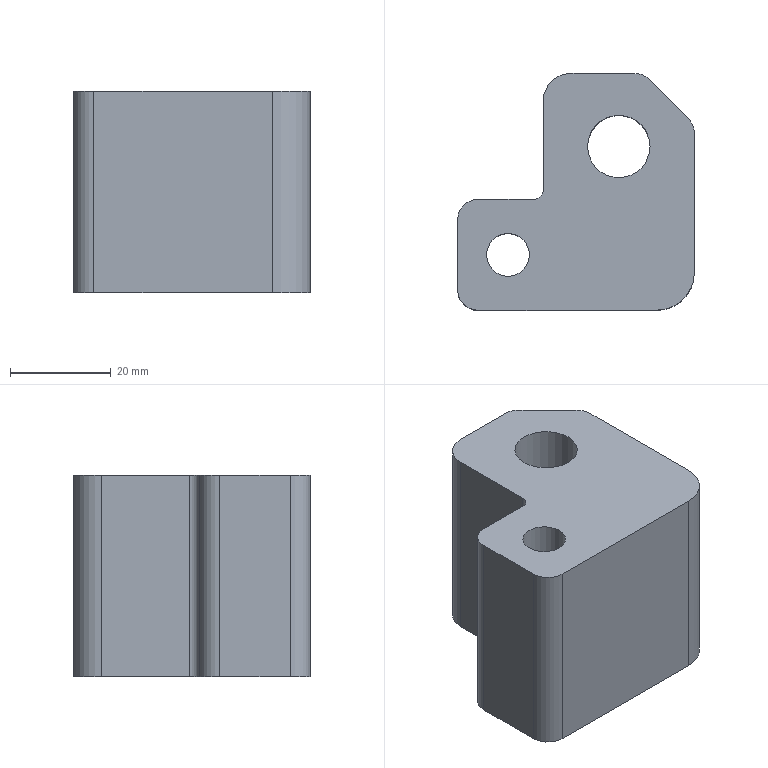Part | NX | features PS-7 2 | 1 solid | 20 faces | box 47 x 47 x 40 mm | volume 59988 mm3 | plane 10 | cylinder 10 | commonest cylinder face diameters 8 x4 4 x1 8.5 x1 11 x1 12.4 x1 14.5 x1
STEP:
#1=CARTESIAN_POINT('',(2465.297,-809.449,860.716));
#2=VERTEX_POINT('',#1);
#3=CARTESIAN_POINT('',(2459.097,-809.449,860.716));
#4=DIRECTION('',(0.,0.,1.));
#5=DIRECTION('',(1.,0.,0.));
#6=AXIS2_PLACEMENT_3D('',#3,#4,#5);
#7=CIRCLE('',#6,6.2);
#8=EDGE_CURVE('',#2,#2,#7,.T.);
#9=ORIENTED_EDGE('',*,*,#8,.T.);
#10=EDGE_LOOP('',(#9));
#11=FACE_BOUND('',#10,.T.);
#12=CARTESIAN_POINT('',(2444.347,-830.949,860.716));
#13=VERTEX_POINT('',#12);
#14=CARTESIAN_POINT('',(2437.097,-830.949,860.716));
#15=DIRECTION('',(0.,0.,1.));
#16=DIRECTION('',(1.,0.,0.));
#17=AXIS2_PLACEMENT_3D('',#14,#15,#16);
#18=CIRCLE('',#17,7.25);
#19=EDGE_CURVE('',#13,#13,#18,.T.);
#20=ORIENTED_EDGE('',*,*,#19,.T.);
#21=EDGE_LOOP('',(#20));
#22=FACE_BOUND('',#21,.T.);
#23=CARTESIAN_POINT('',(2474.097,-834.449,860.716));
#24=VERTEX_POINT('',#23);
#25=CARTESIAN_POINT('',(2466.597,-841.949,860.716));
#26=VERTEX_POINT('',#25);
#27=CARTESIAN_POINT('',(2466.597,-834.449,860.716));
#28=DIRECTION('',(0.,0.,1.));
#29=DIRECTION('',(1.,0.,0.));
#30=AXIS2_PLACEMENT_3D('',#27,#28,#29);
#31=CIRCLE('',#30,7.5);
#32=EDGE_CURVE('',#24,#26,#31,.F.);
#33=ORIENTED_EDGE('',*,*,#32,.T.);
#34=CARTESIAN_POINT('',(2431.097,-841.949,860.716));
#35=VERTEX_POINT('',#34);
#36=CARTESIAN_POINT('',(0.,-841.949,860.716));
#37=DIRECTION('',(1.,0.,0.));
#38=VECTOR('',#37,1000.);
#39=LINE('',#36,#38);
#40=EDGE_CURVE('',#35,#26,#39,.T.);
#41=ORIENTED_EDGE('',*,*,#40,.F.);
#42=CARTESIAN_POINT('',(2427.097,-837.949,860.716));
#43=VERTEX_POINT('',#42);
#44=CARTESIAN_POINT('',(2431.097,-837.949,860.716));
#45=DIRECTION('',(0.,0.,1.));
#46=DIRECTION('',(1.,0.,0.));
#47=AXIS2_PLACEMENT_3D('',#44,#45,#46);
#48=CIRCLE('',#47,4.);
#49=EDGE_CURVE('',#43,#35,#48,.T.);
#50=ORIENTED_EDGE('',*,*,#49,.F.);
#51=CARTESIAN_POINT('',(2427.097,-823.949,860.716));
#52=VERTEX_POINT('',#51);
#53=CARTESIAN_POINT('',(2427.097,-800.449,860.716));
#54=DIRECTION('',(0.,1.,0.));
#55=VECTOR('',#54,1000.);
#56=LINE('',#53,#55);
#57=EDGE_CURVE('',#43,#52,#56,.T.);
#58=ORIENTED_EDGE('',*,*,#57,.T.);
#59=CARTESIAN_POINT('',(2431.097,-819.949,860.716));
#60=VERTEX_POINT('',#59);
#61=CARTESIAN_POINT('',(2431.097,-823.949,860.716));
#62=DIRECTION('',(0.,0.,1.));
#63=DIRECTION('',(1.,0.,0.));
#64=AXIS2_PLACEMENT_3D('',#61,#62,#63);
#65=CIRCLE('',#64,4.);
#66=EDGE_CURVE('',#52,#60,#65,.F.);
#67=ORIENTED_EDGE('',*,*,#66,.T.);
#68=CARTESIAN_POINT('',(2442.097,-819.949,860.716));
#69=VERTEX_POINT('',#68);
#70=CARTESIAN_POINT('',(2437.597,-819.949,860.716));
#71=DIRECTION('',(-1.,0.,0.));
#72=VECTOR('',#71,1000.);
#73=LINE('',#70,#72);
#74=EDGE_CURVE('',#69,#60,#73,.T.);
#75=ORIENTED_EDGE('',*,*,#74,.F.);
#76=CARTESIAN_POINT('',(2444.097,-817.949,860.716));
#77=VERTEX_POINT('',#76);
#78=CARTESIAN_POINT('',(2442.097,-817.949,860.716));
#79=DIRECTION('',(0.,0.,1.));
#80=DIRECTION('',(1.,0.,0.));
#81=AXIS2_PLACEMENT_3D('',#78,#79,#80);
#82=CIRCLE('',#81,2.);
#83=EDGE_CURVE('',#77,#69,#82,.F.);
#84=ORIENTED_EDGE('',*,*,#83,.F.);
#85=CARTESIAN_POINT('',(2444.097,-800.449,860.716));
#86=VERTEX_POINT('',#85);
#87=CARTESIAN_POINT('',(2444.097,-800.449,860.716));
#88=DIRECTION('',(0.,1.,0.));
#89=VECTOR('',#88,1000.);
#90=LINE('',#87,#89);
#91=EDGE_CURVE('',#77,#86,#90,.T.);
#92=ORIENTED_EDGE('',*,*,#91,.T.);
#93=CARTESIAN_POINT('',(2449.597,-794.949,860.716));
#94=VERTEX_POINT('',#93);
#95=CARTESIAN_POINT('',(2449.597,-800.449,860.716));
#96=DIRECTION('',(0.,0.,1.));
#97=DIRECTION('',(1.,0.,0.));
#98=AXIS2_PLACEMENT_3D('',#95,#96,#97);
#99=CIRCLE('',#98,5.5);
#100=EDGE_CURVE('',#86,#94,#99,.F.);
#101=ORIENTED_EDGE('',*,*,#100,.T.);
#102=CARTESIAN_POINT('',(2462.269,-794.949,860.716));
#103=VERTEX_POINT('',#102);
#104=CARTESIAN_POINT('',(0.,-794.949,860.716));
#105=DIRECTION('',(-1.,0.,0.));
#106=VECTOR('',#105,1000.);
#107=LINE('',#104,#106);
#108=EDGE_CURVE('',#103,#94,#107,.T.);
#109=ORIENTED_EDGE('',*,*,#108,.F.);
#110=CARTESIAN_POINT('',(2465.097,-796.12,860.716));
#111=VERTEX_POINT('',#110);
#112=CARTESIAN_POINT('',(2462.269,-798.949,860.716));
#113=DIRECTION('',(0.,0.,1.));
#114=DIRECTION('',(1.,0.,0.));
#115=AXIS2_PLACEMENT_3D('',#112,#113,#114);
#116=CIRCLE('',#115,4.);
#117=EDGE_CURVE('',#103,#111,#116,.F.);
#118=ORIENTED_EDGE('',*,*,#117,.T.);
#119=CARTESIAN_POINT('',(2472.926,-803.949,860.716));
#120=VERTEX_POINT('',#119);
#121=CARTESIAN_POINT('',(834.488,834.488,860.716));
#122=DIRECTION('',(-0.7071,0.7071,0.));
#123=VECTOR('',#122,1000.);
#124=LINE('',#121,#123);
#125=EDGE_CURVE('',#120,#111,#124,.T.);
#126=ORIENTED_EDGE('',*,*,#125,.F.);
#127=CARTESIAN_POINT('',(2474.097,-806.777,860.716));
#128=VERTEX_POINT('',#127);
#129=CARTESIAN_POINT('',(2470.097,-806.777,860.716));
#130=DIRECTION('',(0.,0.,1.));
#131=DIRECTION('',(1.,0.,0.));
#132=AXIS2_PLACEMENT_3D('',#129,#130,#131);
#133=CIRCLE('',#132,4.);
#134=EDGE_CURVE('',#128,#120,#133,.T.);
#135=ORIENTED_EDGE('',*,*,#134,.F.);
#136=CARTESIAN_POINT('',(2474.097,-834.449,860.716));
#137=DIRECTION('',(0.,-1.,0.));
#138=VECTOR('',#137,1000.);
#139=LINE('',#136,#138);
#140=EDGE_CURVE('',#128,#24,#139,.T.);
#141=ORIENTED_EDGE('',*,*,#140,.T.);
#142=EDGE_LOOP('',(#33,#41,#50,#58,#67,#75,#84,#92,#101,#109,#118,#126,#135,#141));
#143=FACE_BOUND('',#142,.T.);
#144=CARTESIAN_POINT('',(0.,0.,860.716));
#145=DIRECTION('',(0.,0.,1.));
#146=DIRECTION('',(1.,0.,0.));
#147=AXIS2_PLACEMENT_3D('',#144,#145,#146);
#148=PLANE('',#147);
#149=ADVANCED_FACE('',(#11,#22,#143),#148,.F.);
#150=ORIENTED_EDGE('',*,*,#91,.F.);
#151=CARTESIAN_POINT('',(2444.097,-817.949,900.716));
#152=VERTEX_POINT('',#151);
#153=CARTESIAN_POINT('',(2444.097,-817.949,830.716));
#154=DIRECTION('',(0.,0.,1.));
#155=VECTOR('',#154,1000.);
#156=LINE('',#153,#155);
#157=EDGE_CURVE('',#77,#152,#156,.T.);
#158=ORIENTED_EDGE('',*,*,#157,.T.);
#159=CARTESIAN_POINT('',(2444.097,-800.449,900.716));
#160=VERTEX_POINT('',#159);
#161=CARTESIAN_POINT('',(2444.097,-800.449,900.716));
#162=DIRECTION('',(0.,1.,0.));
#163=VECTOR('',#162,1000.);
#164=LINE('',#161,#163);
#165=EDGE_CURVE('',#152,#160,#164,.T.);
#166=ORIENTED_EDGE('',*,*,#165,.T.);
#167=CARTESIAN_POINT('',(2444.097,-800.449,830.716));
#168=DIRECTION('',(0.,0.,1.));
#169=VECTOR('',#168,1000.);
#170=LINE('',#167,#169);
#171=EDGE_CURVE('',#160,#86,#170,.F.);
#172=ORIENTED_EDGE('',*,*,#171,.T.);
#173=EDGE_LOOP('',(#150,#158,#166,#172));
#174=FACE_BOUND('',#173,.T.);
#175=CARTESIAN_POINT('',(2444.097,-800.449,830.716));
#176=DIRECTION('',(-1.,0.,0.));
#177=DIRECTION('',(0.,0.,1.));
#178=AXIS2_PLACEMENT_3D('',#175,#176,#177);
#179=PLANE('',#178);
#180=ADVANCED_FACE('',(#174),#179,.T.);
#181=CARTESIAN_POINT('',(2431.097,-841.949,900.716));
#182=VERTEX_POINT('',#181);
#183=CARTESIAN_POINT('',(2466.597,-841.949,900.716));
#184=VERTEX_POINT('',#183);
#185=CARTESIAN_POINT('',(0.,-841.949,900.716));
#186=DIRECTION('',(1.,0.,0.));
#187=VECTOR('',#186,1000.);
#188=LINE('',#185,#187);
#189=EDGE_CURVE('',#182,#184,#188,.T.);
#190=ORIENTED_EDGE('',*,*,#189,.F.);
#191=CARTESIAN_POINT('',(2431.097,-841.949,830.716));
#192=DIRECTION('',(0.,0.,-1.));
#193=VECTOR('',#192,1000.);
#194=LINE('',#191,#193);
#195=EDGE_CURVE('',#182,#35,#194,.T.);
#196=ORIENTED_EDGE('',*,*,#195,.T.);
#197=ORIENTED_EDGE('',*,*,#40,.T.);
#198=CARTESIAN_POINT('',(2466.597,-841.949,830.716));
#199=DIRECTION('',(0.,0.,1.));
#200=VECTOR('',#199,1000.);
#201=LINE('',#198,#200);
#202=EDGE_CURVE('',#184,#26,#201,.F.);
#203=ORIENTED_EDGE('',*,*,#202,.F.);
#204=EDGE_LOOP('',(#190,#196,#197,#203));
#205=FACE_BOUND('',#204,.T.);
#206=CARTESIAN_POINT('',(2449.597,-841.949,830.716));
#207=DIRECTION('',(0.,-1.,0.));
#208=DIRECTION('',(0.,0.,-1.));
#209=AXIS2_PLACEMENT_3D('',#206,#207,#208);
#210=PLANE('',#209);
#211=ADVANCED_FACE('',(#205),#210,.T.);
#212=ORIENTED_EDGE('',*,*,#202,.T.);
#213=ORIENTED_EDGE('',*,*,#32,.F.);
#214=CARTESIAN_POINT('',(2474.097,-834.449,900.716));
#215=VERTEX_POINT('',#214);
#216=CARTESIAN_POINT('',(2474.097,-834.449,830.716));
#217=DIRECTION('',(0.,0.,-1.));
#218=VECTOR('',#217,1000.);
#219=LINE('',#216,#218);
#220=EDGE_CURVE('',#215,#24,#219,.T.);
#221=ORIENTED_EDGE('',*,*,#220,.F.);
#222=CARTESIAN_POINT('',(2466.597,-834.449,900.716));
#223=DIRECTION('',(0.,0.,1.));
#224=DIRECTION('',(1.,0.,0.));
#225=AXIS2_PLACEMENT_3D('',#222,#223,#224);
#226=CIRCLE('',#225,7.5);
#227=EDGE_CURVE('',#215,#184,#226,.F.);
#228=ORIENTED_EDGE('',*,*,#227,.T.);
#229=EDGE_LOOP('',(#212,#213,#221,#228));
#230=FACE_BOUND('',#229,.T.);
#231=CARTESIAN_POINT('',(2466.597,-834.449,830.716));
#232=DIRECTION('',(0.,0.,1.));
#233=DIRECTION('',(1.,0.,0.));
#234=AXIS2_PLACEMENT_3D('',#231,#232,#233);
#235=CYLINDRICAL_SURFACE('',#234,7.5);
#236=ADVANCED_FACE('',(#230),#235,.T.);
#237=ORIENTED_EDGE('',*,*,#220,.T.);
#238=ORIENTED_EDGE('',*,*,#140,.F.);
#239=CARTESIAN_POINT('',(2474.097,-806.777,900.716));
#240=VERTEX_POINT('',#239);
#241=CARTESIAN_POINT('',(2474.097,-806.777,830.716));
#242=DIRECTION('',(0.,0.,1.));
#243=VECTOR('',#242,1000.);
#244=LINE('',#241,#243);
#245=EDGE_CURVE('',#240,#128,#244,.F.);
#246=ORIENTED_EDGE('',*,*,#245,.F.);
#247=CARTESIAN_POINT('',(2474.097,-834.449,900.716));
#248=DIRECTION('',(0.,-1.,0.));
#249=VECTOR('',#248,1000.);
#250=LINE('',#247,#249);
#251=EDGE_CURVE('',#240,#215,#250,.T.);
#252=ORIENTED_EDGE('',*,*,#251,.T.);
#253=EDGE_LOOP('',(#237,#238,#246,#252));
#254=FACE_BOUND('',#253,.T.);
#255=CARTESIAN_POINT('',(2474.097,-834.449,830.716));
#256=DIRECTION('',(1.,0.,0.));
#257=DIRECTION('',(0.,0.,-1.));
#258=AXIS2_PLACEMENT_3D('',#255,#256,#257);
#259=PLANE('',#258);
#260=ADVANCED_FACE('',(#254),#259,.T.);
#261=ORIENTED_EDGE('',*,*,#245,.T.);
#262=ORIENTED_EDGE('',*,*,#134,.T.);
#263=CARTESIAN_POINT('',(2472.926,-803.949,900.716));
#264=VERTEX_POINT('',#263);
#265=CARTESIAN_POINT('',(2472.926,-803.949,830.716));
#266=DIRECTION('',(0.,0.,1.));
#267=VECTOR('',#266,1000.);
#268=LINE('',#265,#267);
#269=EDGE_CURVE('',#264,#120,#268,.F.);
#270=ORIENTED_EDGE('',*,*,#269,.F.);
#271=CARTESIAN_POINT('',(2470.097,-806.777,900.716));
#272=DIRECTION('',(0.,0.,1.));
#273=DIRECTION('',(1.,0.,0.));
#274=AXIS2_PLACEMENT_3D('',#271,#272,#273);
#275=CIRCLE('',#274,4.);
#276=EDGE_CURVE('',#264,#240,#275,.F.);
#277=ORIENTED_EDGE('',*,*,#276,.T.);
#278=EDGE_LOOP('',(#261,#262,#270,#277));
#279=FACE_BOUND('',#278,.T.);
#280=CARTESIAN_POINT('',(2470.097,-806.777,830.716));
#281=DIRECTION('',(0.,0.,1.));
#282=DIRECTION('',(1.,0.,0.));
#283=AXIS2_PLACEMENT_3D('',#280,#281,#282);
#284=CYLINDRICAL_SURFACE('',#283,4.);
#285=ADVANCED_FACE('',(#279),#284,.T.);
#286=ORIENTED_EDGE('',*,*,#269,.T.);
#287=ORIENTED_EDGE('',*,*,#125,.T.);
#288=CARTESIAN_POINT('',(2465.097,-796.12,900.716));
#289=VERTEX_POINT('',#288);
#290=CARTESIAN_POINT('',(2465.097,-796.12,830.716));
#291=DIRECTION('',(0.,0.,1.));
#292=VECTOR('',#291,1000.);
#293=LINE('',#290,#292);
#294=EDGE_CURVE('',#289,#111,#293,.F.);
#295=ORIENTED_EDGE('',*,*,#294,.F.);
#296=CARTESIAN_POINT('',(2472.926,-803.949,900.716));
#297=DIRECTION('',(0.7071,-0.7071,0.));
#298=VECTOR('',#297,1000.);
#299=LINE('',#296,#298);
#300=EDGE_CURVE('',#289,#264,#299,.T.);
#301=ORIENTED_EDGE('',*,*,#300,.T.);
#302=EDGE_LOOP('',(#286,#287,#295,#301));
#303=FACE_BOUND('',#302,.T.);
#304=CARTESIAN_POINT('',(2472.926,-803.949,830.716));
#305=DIRECTION('',(0.7071,0.7071,0.));
#306=DIRECTION('',(-0.7071,0.7071,0.));
#307=AXIS2_PLACEMENT_3D('',#304,#305,#306);
#308=PLANE('',#307);
#309=ADVANCED_FACE('',(#303),#308,.T.);
#310=ORIENTED_EDGE('',*,*,#294,.T.);
#311=ORIENTED_EDGE('',*,*,#117,.F.);
#312=CARTESIAN_POINT('',(2462.269,-794.949,900.716));
#313=VERTEX_POINT('',#312);
#314=CARTESIAN_POINT('',(2462.269,-794.949,830.716));
#315=DIRECTION('',(0.,0.,1.));
#316=VECTOR('',#315,1000.);
#317=LINE('',#314,#316);
#318=EDGE_CURVE('',#313,#103,#317,.F.);
#319=ORIENTED_EDGE('',*,*,#318,.F.);
#320=CARTESIAN_POINT('',(2462.269,-798.949,900.716));
#321=DIRECTION('',(0.,0.,1.));
#322=DIRECTION('',(1.,0.,0.));
#323=AXIS2_PLACEMENT_3D('',#320,#321,#322);
#324=CIRCLE('',#323,4.);
#325=EDGE_CURVE('',#313,#289,#324,.F.);
#326=ORIENTED_EDGE('',*,*,#325,.T.);
#327=EDGE_LOOP('',(#310,#311,#319,#326));
#328=FACE_BOUND('',#327,.T.);
#329=CARTESIAN_POINT('',(2462.269,-798.949,830.716));
#330=DIRECTION('',(0.,0.,1.));
#331=DIRECTION('',(1.,0.,0.));
#332=AXIS2_PLACEMENT_3D('',#329,#330,#331);
#333=CYLINDRICAL_SURFACE('',#332,4.);
#334=ADVANCED_FACE('',(#328),#333,.T.);
#335=ORIENTED_EDGE('',*,*,#318,.T.);
#336=ORIENTED_EDGE('',*,*,#108,.T.);
#337=CARTESIAN_POINT('',(2449.597,-794.949,900.716));
#338=VERTEX_POINT('',#337);
#339=CARTESIAN_POINT('',(2449.597,-794.949,830.716));
#340=DIRECTION('',(0.,0.,1.));
#341=VECTOR('',#340,1000.);
#342=LINE('',#339,#341);
#343=EDGE_CURVE('',#338,#94,#342,.F.);
#344=ORIENTED_EDGE('',*,*,#343,.F.);
#345=CARTESIAN_POINT('',(2462.269,-794.949,900.716));
#346=DIRECTION('',(1.,0.,0.));
#347=VECTOR('',#346,1000.);
#348=LINE('',#345,#347);
#349=EDGE_CURVE('',#338,#313,#348,.T.);
#350=ORIENTED_EDGE('',*,*,#349,.T.);
#351=EDGE_LOOP('',(#335,#336,#344,#350));
#352=FACE_BOUND('',#351,.T.);
#353=CARTESIAN_POINT('',(2462.269,-794.949,830.716));
#354=DIRECTION('',(0.,1.,0.));
#355=DIRECTION('',(0.,0.,1.));
#356=AXIS2_PLACEMENT_3D('',#353,#354,#355);
#357=PLANE('',#356);
#358=ADVANCED_FACE('',(#352),#357,.T.);
#359=ORIENTED_EDGE('',*,*,#343,.T.);
#360=ORIENTED_EDGE('',*,*,#100,.F.);
#361=ORIENTED_EDGE('',*,*,#171,.F.);
#362=CARTESIAN_POINT('',(2449.597,-800.449,900.716));
#363=DIRECTION('',(0.,0.,1.));
#364=DIRECTION('',(1.,0.,0.));
#365=AXIS2_PLACEMENT_3D('',#362,#363,#364);
#366=CIRCLE('',#365,5.5);
#367=EDGE_CURVE('',#160,#338,#366,.F.);
#368=ORIENTED_EDGE('',*,*,#367,.T.);
#369=EDGE_LOOP('',(#359,#360,#361,#368));
#370=FACE_BOUND('',#369,.T.);
#371=CARTESIAN_POINT('',(2449.597,-800.449,830.716));
#372=DIRECTION('',(0.,0.,1.));
#373=DIRECTION('',(1.,0.,0.));
#374=AXIS2_PLACEMENT_3D('',#371,#372,#373);
#375=CYLINDRICAL_SURFACE('',#374,5.5);
#376=ADVANCED_FACE('',(#370),#375,.T.);
#377=ORIENTED_EDGE('',*,*,#57,.F.);
#378=CARTESIAN_POINT('',(2427.097,-837.949,900.716));
#379=VERTEX_POINT('',#378);
#380=CARTESIAN_POINT('',(2427.097,-837.949,830.716));
#381=DIRECTION('',(0.,0.,1.));
#382=VECTOR('',#381,1000.);
#383=LINE('',#380,#382);
#384=EDGE_CURVE('',#43,#379,#383,.T.);
#385=ORIENTED_EDGE('',*,*,#384,.T.);
#386=CARTESIAN_POINT('',(2427.097,-823.949,900.716));
#387=VERTEX_POINT('',#386);
#388=CARTESIAN_POINT('',(2427.097,-800.449,900.716));
#389=DIRECTION('',(0.,1.,0.));
#390=VECTOR('',#389,1000.);
#391=LINE('',#388,#390);
#392=EDGE_CURVE('',#379,#387,#391,.T.);
#393=ORIENTED_EDGE('',*,*,#392,.T.);
#394=CARTESIAN_POINT('',(2427.097,-823.949,830.716));
#395=DIRECTION('',(0.,0.,1.));
#396=VECTOR('',#395,1000.);
#397=LINE('',#394,#396);
#398=EDGE_CURVE('',#387,#52,#397,.F.);
#399=ORIENTED_EDGE('',*,*,#398,.T.);
#400=EDGE_LOOP('',(#377,#385,#393,#399));
#401=FACE_BOUND('',#400,.T.);
#402=CARTESIAN_POINT('',(2427.097,-800.449,830.716));
#403=DIRECTION('',(-1.,0.,0.));
#404=DIRECTION('',(0.,0.,1.));
#405=AXIS2_PLACEMENT_3D('',#402,#403,#404);
#406=PLANE('',#405);
#407=ADVANCED_FACE('',(#401),#406,.T.);
#408=CARTESIAN_POINT('',(2431.097,-819.949,900.716));
#409=VERTEX_POINT('',#408);
#410=CARTESIAN_POINT('',(2442.097,-819.949,900.716));
#411=VERTEX_POINT('',#410);
#412=CARTESIAN_POINT('',(0.,-819.949,900.716));
#413=DIRECTION('',(1.,0.,0.));
#414=VECTOR('',#413,1000.);
#415=LINE('',#412,#414);
#416=EDGE_CURVE('',#409,#411,#415,.T.);
#417=ORIENTED_EDGE('',*,*,#416,.T.);
#418=CARTESIAN_POINT('',(2442.097,-819.949,875.716));
#419=DIRECTION('',(0.,0.,-1.));
#420=VECTOR('',#419,1000.);
#421=LINE('',#418,#420);
#422=EDGE_CURVE('',#411,#69,#421,.T.);
#423=ORIENTED_EDGE('',*,*,#422,.T.);
#424=ORIENTED_EDGE('',*,*,#74,.T.);
#425=CARTESIAN_POINT('',(2431.097,-819.949,875.716));
#426=DIRECTION('',(0.,0.,-1.));
#427=VECTOR('',#426,1000.);
#428=LINE('',#425,#427);
#429=EDGE_CURVE('',#60,#409,#428,.F.);
#430=ORIENTED_EDGE('',*,*,#429,.T.);
#431=EDGE_LOOP('',(#417,#423,#424,#430));
#432=FACE_BOUND('',#431,.T.);
#433=CARTESIAN_POINT('',(2437.597,-819.949,875.716));
#434=DIRECTION('',(0.,-1.,0.));
#435=DIRECTION('',(0.,0.,-1.));
#436=AXIS2_PLACEMENT_3D('',#433,#434,#435);
#437=PLANE('',#436);
#438=ADVANCED_FACE('',(#432),#437,.F.);
#439=ORIENTED_EDGE('',*,*,#83,.T.);
#440=ORIENTED_EDGE('',*,*,#422,.F.);
#441=CARTESIAN_POINT('',(2442.097,-817.949,900.716));
#442=DIRECTION('',(0.,0.,1.));
#443=DIRECTION('',(1.,0.,0.));
#444=AXIS2_PLACEMENT_3D('',#441,#442,#443);
#445=CIRCLE('',#444,2.);
#446=EDGE_CURVE('',#152,#411,#445,.F.);
#447=ORIENTED_EDGE('',*,*,#446,.F.);
#448=ORIENTED_EDGE('',*,*,#157,.F.);
#449=EDGE_LOOP('',(#439,#440,#447,#448));
#450=FACE_BOUND('',#449,.T.);
#451=CARTESIAN_POINT('',(2442.097,-817.949,830.716));
#452=DIRECTION('',(0.,0.,1.));
#453=DIRECTION('',(1.,0.,0.));
#454=AXIS2_PLACEMENT_3D('',#451,#452,#453);
#455=CYLINDRICAL_SURFACE('',#454,2.);
#456=ADVANCED_FACE('',(#450),#455,.F.);
#457=CARTESIAN_POINT('',(2431.097,-837.949,900.716));
#458=DIRECTION('',(0.,0.,1.));
#459=DIRECTION('',(1.,0.,0.));
#460=AXIS2_PLACEMENT_3D('',#457,#458,#459);
#461=CIRCLE('',#460,4.);
#462=EDGE_CURVE('',#379,#182,#461,.T.);
#463=ORIENTED_EDGE('',*,*,#462,.F.);
#464=ORIENTED_EDGE('',*,*,#384,.F.);
#465=ORIENTED_EDGE('',*,*,#49,.T.);
#466=ORIENTED_EDGE('',*,*,#195,.F.);
#467=EDGE_LOOP('',(#463,#464,#465,#466));
#468=FACE_BOUND('',#467,.T.);
#469=CARTESIAN_POINT('',(2431.097,-837.949,830.716));
#470=DIRECTION('',(0.,0.,-1.));
#471=DIRECTION('',(-1.,0.,0.));
#472=AXIS2_PLACEMENT_3D('',#469,#470,#471);
#473=CYLINDRICAL_SURFACE('',#472,4.);
#474=ADVANCED_FACE('',(#468),#473,.T.);
#475=ORIENTED_EDGE('',*,*,#66,.F.);
#476=ORIENTED_EDGE('',*,*,#398,.F.);
#477=CARTESIAN_POINT('',(2431.097,-823.949,900.716));
#478=DIRECTION('',(0.,0.,1.));
#479=DIRECTION('',(1.,0.,0.));
#480=AXIS2_PLACEMENT_3D('',#477,#478,#479);
#481=CIRCLE('',#480,4.);
#482=EDGE_CURVE('',#387,#409,#481,.F.);
#483=ORIENTED_EDGE('',*,*,#482,.T.);
#484=ORIENTED_EDGE('',*,*,#429,.F.);
#485=EDGE_LOOP('',(#475,#476,#483,#484));
#486=FACE_BOUND('',#485,.T.);
#487=CARTESIAN_POINT('',(2431.097,-823.949,875.716));
#488=DIRECTION('',(0.,0.,-1.));
#489=DIRECTION('',(-1.,0.,0.));
#490=AXIS2_PLACEMENT_3D('',#487,#488,#489);
#491=CYLINDRICAL_SURFACE('',#490,4.);
#492=ADVANCED_FACE('',(#486),#491,.T.);
#493=CARTESIAN_POINT('',(2465.297,-809.449,900.716));
#494=VERTEX_POINT('',#493);
#495=CARTESIAN_POINT('',(2459.097,-809.449,900.716));
#496=DIRECTION('',(0.,0.,1.));
#497=DIRECTION('',(1.,0.,0.));
#498=AXIS2_PLACEMENT_3D('',#495,#496,#497);
#499=CIRCLE('',#498,6.2);
#500=EDGE_CURVE('',#494,#494,#499,.F.);
#501=ORIENTED_EDGE('',*,*,#500,.T.);
#502=EDGE_LOOP('',(#501));
#503=FACE_BOUND('',#502,.T.);
#504=CARTESIAN_POINT('',(2441.347,-830.949,900.716));
#505=VERTEX_POINT('',#504);
#506=CARTESIAN_POINT('',(2437.097,-830.949,900.716));
#507=DIRECTION('',(0.,0.,1.));
#508=DIRECTION('',(1.,0.,0.));
#509=AXIS2_PLACEMENT_3D('',#506,#507,#508);
#510=CIRCLE('',#509,4.25);
#511=EDGE_CURVE('',#505,#505,#510,.T.);
#512=ORIENTED_EDGE('',*,*,#511,.F.);
#513=EDGE_LOOP('',(#512));
#514=FACE_BOUND('',#513,.T.);
#515=ORIENTED_EDGE('',*,*,#189,.T.);
#516=ORIENTED_EDGE('',*,*,#227,.F.);
#517=ORIENTED_EDGE('',*,*,#251,.F.);
#518=ORIENTED_EDGE('',*,*,#276,.F.);
#519=ORIENTED_EDGE('',*,*,#300,.F.);
#520=ORIENTED_EDGE('',*,*,#325,.F.);
#521=ORIENTED_EDGE('',*,*,#349,.F.);
#522=ORIENTED_EDGE('',*,*,#367,.F.);
#523=ORIENTED_EDGE('',*,*,#165,.F.);
#524=ORIENTED_EDGE('',*,*,#446,.T.);
#525=ORIENTED_EDGE('',*,*,#416,.F.);
#526=ORIENTED_EDGE('',*,*,#482,.F.);
#527=ORIENTED_EDGE('',*,*,#392,.F.);
#528=ORIENTED_EDGE('',*,*,#462,.T.);
#529=EDGE_LOOP('',(#515,#516,#517,#518,#519,#520,#521,#522,#523,#524,#525,#526,#527,#528));
#530=FACE_BOUND('',#529,.T.);
#531=CARTESIAN_POINT('',(0.,0.,900.716));
#532=DIRECTION('',(0.,0.,1.));
#533=DIRECTION('',(1.,0.,0.));
#534=AXIS2_PLACEMENT_3D('',#531,#532,#533);
#535=PLANE('',#534);
#536=ADVANCED_FACE('',(#503,#514,#530),#535,.T.);
#537=CARTESIAN_POINT('',(2437.097,-823.699,871.716));
#538=VERTEX_POINT('',#537);
#539=CARTESIAN_POINT('',(2437.097,-830.949,871.716));
#540=DIRECTION('',(0.,0.,-1.));
#541=DIRECTION('',(0.,1.,0.));
#542=AXIS2_PLACEMENT_3D('',#539,#540,#541);
#543=CIRCLE('',#542,7.25);
#544=EDGE_CURVE('',#538,#538,#543,.F.);
#545=ORIENTED_EDGE('',*,*,#544,.T.);
#546=EDGE_LOOP('',(#545));
#547=FACE_BOUND('',#546,.T.);
#548=ORIENTED_EDGE('',*,*,#19,.F.);
#549=EDGE_LOOP('',(#548));
#550=FACE_BOUND('',#549,.T.);
#551=CARTESIAN_POINT('',(2437.097,-830.949,871.716));
#552=DIRECTION('',(0.,0.,-1.));
#553=DIRECTION('',(-1.,0.,0.));
#554=AXIS2_PLACEMENT_3D('',#551,#552,#553);
#555=CYLINDRICAL_SURFACE('',#554,7.25);
#556=ADVANCED_FACE('',(#547,#550),#555,.F.);
#557=ORIENTED_EDGE('',*,*,#511,.T.);
#558=EDGE_LOOP('',(#557));
#559=FACE_BOUND('',#558,.T.);
#560=CARTESIAN_POINT('',(2432.847,-830.949,871.716));
#561=VERTEX_POINT('',#560);
#562=CARTESIAN_POINT('',(2437.097,-830.949,871.716));
#563=DIRECTION('',(0.,0.,-1.));
#564=DIRECTION('',(-1.,0.,0.));
#565=AXIS2_PLACEMENT_3D('',#562,#563,#564);
#566=CIRCLE('',#565,4.25);
#567=EDGE_CURVE('',#561,#561,#566,.T.);
#568=ORIENTED_EDGE('',*,*,#567,.T.);
#569=EDGE_LOOP('',(#568));
#570=FACE_BOUND('',#569,.T.);
#571=CARTESIAN_POINT('',(2437.097,-830.949,891.716));
#572=DIRECTION('',(0.,0.,-1.));
#573=DIRECTION('',(-1.,0.,0.));
#574=AXIS2_PLACEMENT_3D('',#571,#572,#573);
#575=CYLINDRICAL_SURFACE('',#574,4.25);
#576=ADVANCED_FACE('',(#559,#570),#575,.F.);
#577=ORIENTED_EDGE('',*,*,#567,.F.);
#578=EDGE_LOOP('',(#577));
#579=FACE_BOUND('',#578,.T.);
#580=ORIENTED_EDGE('',*,*,#544,.F.);
#581=EDGE_LOOP('',(#580));
#582=FACE_BOUND('',#581,.T.);
#583=CARTESIAN_POINT('',(2437.097,-830.949,871.716));
#584=DIRECTION('',(0.,0.,-1.));
#585=DIRECTION('',(-1.,0.,0.));
#586=AXIS2_PLACEMENT_3D('',#583,#584,#585);
#587=PLANE('',#586);
#588=ADVANCED_FACE('',(#579,#582),#587,.T.);
#589=ORIENTED_EDGE('',*,*,#500,.F.);
#590=EDGE_LOOP('',(#589));
#591=FACE_BOUND('',#590,.T.);
#592=ORIENTED_EDGE('',*,*,#8,.F.);
#593=EDGE_LOOP('',(#592));
#594=FACE_BOUND('',#593,.T.);
#595=CARTESIAN_POINT('',(2459.097,-809.449,940.716));
#596=DIRECTION('',(0.,0.,-1.));
#597=DIRECTION('',(-1.,0.,0.));
#598=AXIS2_PLACEMENT_3D('',#595,#596,#597);
#599=CYLINDRICAL_SURFACE('',#598,6.2);
#600=ADVANCED_FACE('',(#591,#594),#599,.F.);
#601=CLOSED_SHELL('',(#149,#180,#211,#236,#260,#285,#309,#334,#358,#376,#407,#438,#456,#474,#492,#536,#556,#576,#588,#600));
#602=MANIFOLD_SOLID_BREP('',#601);
#603=(LENGTH_UNIT()NAMED_UNIT(*)SI_UNIT(.MILLI.,.METRE.));
#604=UNCERTAINTY_MEASURE_WITH_UNIT(LENGTH_MEASURE(0.00001),#603,'','');
#605=(NAMED_UNIT(*)PLANE_ANGLE_UNIT()SI_UNIT($,.RADIAN.));
#606=(NAMED_UNIT(*)SI_UNIT($,.STERADIAN.)SOLID_ANGLE_UNIT());
#607=(GEOMETRIC_REPRESENTATION_CONTEXT(3)GLOBAL_UNCERTAINTY_ASSIGNED_CONTEXT((#604))GLOBAL_UNIT_ASSIGNED_CONTEXT((#603,#605,#606))REPRESENTATION_CONTEXT('',''));
#608=ADVANCED_BREP_SHAPE_REPRESENTATION('',(#602),#607);